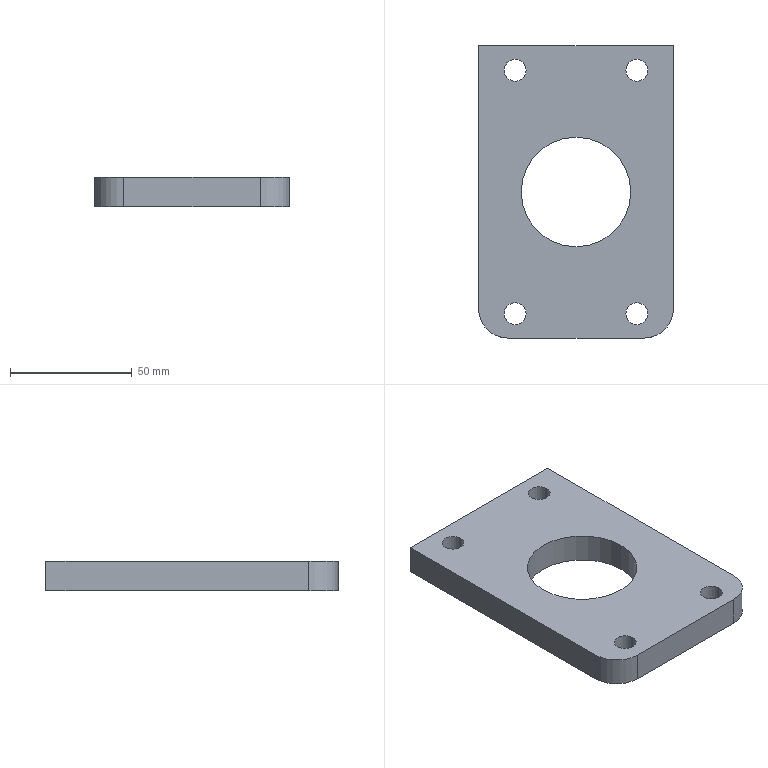Part | SolidWorks | features BaseBody 1 | 1 solid | 18 faces | box 80 x 120 x 12 mm | volume 92320 mm3 | cylinder 12 | plane 6 | commonest cylinder face diameters 9 x8 24 x2 45 x2
STEP:
#1=CARTESIAN_POINT('',(-255.5,-50.,-47.879));
#2=VERTEX_POINT('',#1);
#3=CARTESIAN_POINT('',(-264.5,-50.,-47.879));
#4=VERTEX_POINT('',#3);
#5=CARTESIAN_POINT('',(-260.,-50.,-47.879));
#6=DIRECTION('',(0.,0.,-1.));
#7=DIRECTION('',(-1.,0.,0.));
#8=AXIS2_PLACEMENT_3D('',#5,#6,#7);
#9=CIRCLE('',#8,4.5);
#10=EDGE_CURVE('',#2,#4,#9,.T.);
#11=ORIENTED_EDGE('',*,*,#10,.F.);
#12=CARTESIAN_POINT('',(-255.5,-50.,-59.879));
#13=VERTEX_POINT('',#12);
#14=CARTESIAN_POINT('',(-255.5,-50.,-59.879));
#15=DIRECTION('',(0.,0.,-1.));
#16=VECTOR('',#15,1000.);
#17=LINE('',#14,#16);
#18=EDGE_CURVE('',#2,#13,#17,.T.);
#19=ORIENTED_EDGE('',*,*,#18,.T.);
#20=CARTESIAN_POINT('',(-264.5,-50.,-59.879));
#21=VERTEX_POINT('',#20);
#22=CARTESIAN_POINT('',(-260.,-50.,-59.879));
#23=DIRECTION('',(0.,0.,1.));
#24=DIRECTION('',(-1.,0.,0.));
#25=AXIS2_PLACEMENT_3D('',#22,#23,#24);
#26=CIRCLE('',#25,4.5);
#27=EDGE_CURVE('',#21,#13,#26,.T.);
#28=ORIENTED_EDGE('',*,*,#27,.F.);
#29=CARTESIAN_POINT('',(-264.5,-50.,-59.879));
#30=DIRECTION('',(0.,0.,-1.));
#31=VECTOR('',#30,1000.);
#32=LINE('',#29,#31);
#33=EDGE_CURVE('',#4,#21,#32,.T.);
#34=ORIENTED_EDGE('',*,*,#33,.F.);
#35=EDGE_LOOP('',(#11,#19,#28,#34));
#36=FACE_OUTER_BOUND('',#35,.T.);
#37=CARTESIAN_POINT('',(-260.,-50.,-59.879));
#38=DIRECTION('',(0.,0.,-1.));
#39=DIRECTION('',(-1.,0.,0.));
#40=AXIS2_PLACEMENT_3D('',#37,#38,#39);
#41=CYLINDRICAL_SURFACE('',#40,4.5);
#42=ADVANCED_FACE('',(#36),#41,.F.);
#43=CARTESIAN_POINT('',(-205.5,-50.,-47.879));
#44=VERTEX_POINT('',#43);
#45=CARTESIAN_POINT('',(-214.5,-50.,-47.879));
#46=VERTEX_POINT('',#45);
#47=CARTESIAN_POINT('',(-210.,-50.,-47.879));
#48=DIRECTION('',(0.,0.,-1.));
#49=DIRECTION('',(-1.,0.,0.));
#50=AXIS2_PLACEMENT_3D('',#47,#48,#49);
#51=CIRCLE('',#50,4.5);
#52=EDGE_CURVE('',#44,#46,#51,.T.);
#53=ORIENTED_EDGE('',*,*,#52,.F.);
#54=CARTESIAN_POINT('',(-205.5,-50.,-59.879));
#55=VERTEX_POINT('',#54);
#56=CARTESIAN_POINT('',(-205.5,-50.,-59.879));
#57=DIRECTION('',(0.,0.,-1.));
#58=VECTOR('',#57,1000.);
#59=LINE('',#56,#58);
#60=EDGE_CURVE('',#44,#55,#59,.T.);
#61=ORIENTED_EDGE('',*,*,#60,.T.);
#62=CARTESIAN_POINT('',(-214.5,-50.,-59.879));
#63=VERTEX_POINT('',#62);
#64=CARTESIAN_POINT('',(-210.,-50.,-59.879));
#65=DIRECTION('',(0.,0.,1.));
#66=DIRECTION('',(-1.,0.,0.));
#67=AXIS2_PLACEMENT_3D('',#64,#65,#66);
#68=CIRCLE('',#67,4.5);
#69=EDGE_CURVE('',#63,#55,#68,.T.);
#70=ORIENTED_EDGE('',*,*,#69,.F.);
#71=CARTESIAN_POINT('',(-214.5,-50.,-59.879));
#72=DIRECTION('',(0.,0.,-1.));
#73=VECTOR('',#72,1000.);
#74=LINE('',#71,#73);
#75=EDGE_CURVE('',#46,#63,#74,.T.);
#76=ORIENTED_EDGE('',*,*,#75,.F.);
#77=EDGE_LOOP('',(#53,#61,#70,#76));
#78=FACE_OUTER_BOUND('',#77,.T.);
#79=CARTESIAN_POINT('',(-210.,-50.,-59.879));
#80=DIRECTION('',(0.,0.,-1.));
#81=DIRECTION('',(-1.,0.,0.));
#82=AXIS2_PLACEMENT_3D('',#79,#80,#81);
#83=CYLINDRICAL_SURFACE('',#82,4.5);
#84=ADVANCED_FACE('',(#78),#83,.F.);
#85=CARTESIAN_POINT('',(-212.5,0.,-47.879));
#86=VERTEX_POINT('',#85);
#87=CARTESIAN_POINT('',(-257.5,0.,-47.879));
#88=VERTEX_POINT('',#87);
#89=CARTESIAN_POINT('',(-235.,0.,-47.879));
#90=DIRECTION('',(0.,0.,-1.));
#91=DIRECTION('',(-1.,0.,0.));
#92=AXIS2_PLACEMENT_3D('',#89,#90,#91);
#93=CIRCLE('',#92,22.5);
#94=EDGE_CURVE('',#86,#88,#93,.T.);
#95=ORIENTED_EDGE('',*,*,#94,.F.);
#96=CARTESIAN_POINT('',(-212.5,0.,-59.879));
#97=VERTEX_POINT('',#96);
#98=CARTESIAN_POINT('',(-212.5,0.,-59.879));
#99=DIRECTION('',(0.,0.,-1.));
#100=VECTOR('',#99,1000.);
#101=LINE('',#98,#100);
#102=EDGE_CURVE('',#86,#97,#101,.T.);
#103=ORIENTED_EDGE('',*,*,#102,.T.);
#104=CARTESIAN_POINT('',(-257.5,0.,-59.879));
#105=VERTEX_POINT('',#104);
#106=CARTESIAN_POINT('',(-235.,0.,-59.879));
#107=DIRECTION('',(0.,0.,1.));
#108=DIRECTION('',(-1.,0.,0.));
#109=AXIS2_PLACEMENT_3D('',#106,#107,#108);
#110=CIRCLE('',#109,22.5);
#111=EDGE_CURVE('',#105,#97,#110,.T.);
#112=ORIENTED_EDGE('',*,*,#111,.F.);
#113=CARTESIAN_POINT('',(-257.5,0.,-59.879));
#114=DIRECTION('',(0.,0.,-1.));
#115=VECTOR('',#114,1000.);
#116=LINE('',#113,#115);
#117=EDGE_CURVE('',#88,#105,#116,.T.);
#118=ORIENTED_EDGE('',*,*,#117,.F.);
#119=EDGE_LOOP('',(#95,#103,#112,#118));
#120=FACE_OUTER_BOUND('',#119,.T.);
#121=CARTESIAN_POINT('',(-235.,0.,-59.879));
#122=DIRECTION('',(0.,0.,-1.));
#123=DIRECTION('',(-1.,0.,0.));
#124=AXIS2_PLACEMENT_3D('',#121,#122,#123);
#125=CYLINDRICAL_SURFACE('',#124,22.5);
#126=ADVANCED_FACE('',(#120),#125,.F.);
#127=CARTESIAN_POINT('',(-255.5,50.,-47.879));
#128=VERTEX_POINT('',#127);
#129=CARTESIAN_POINT('',(-264.5,50.,-47.879));
#130=VERTEX_POINT('',#129);
#131=CARTESIAN_POINT('',(-260.,50.,-47.879));
#132=DIRECTION('',(0.,0.,-1.));
#133=DIRECTION('',(-1.,0.,0.));
#134=AXIS2_PLACEMENT_3D('',#131,#132,#133);
#135=CIRCLE('',#134,4.5);
#136=EDGE_CURVE('',#128,#130,#135,.T.);
#137=ORIENTED_EDGE('',*,*,#136,.F.);
#138=CARTESIAN_POINT('',(-255.5,50.,-59.879));
#139=VERTEX_POINT('',#138);
#140=CARTESIAN_POINT('',(-255.5,50.,-59.879));
#141=DIRECTION('',(0.,0.,-1.));
#142=VECTOR('',#141,1000.);
#143=LINE('',#140,#142);
#144=EDGE_CURVE('',#128,#139,#143,.T.);
#145=ORIENTED_EDGE('',*,*,#144,.T.);
#146=CARTESIAN_POINT('',(-264.5,50.,-59.879));
#147=VERTEX_POINT('',#146);
#148=CARTESIAN_POINT('',(-260.,50.,-59.879));
#149=DIRECTION('',(0.,0.,1.));
#150=DIRECTION('',(-1.,0.,0.));
#151=AXIS2_PLACEMENT_3D('',#148,#149,#150);
#152=CIRCLE('',#151,4.5);
#153=EDGE_CURVE('',#147,#139,#152,.T.);
#154=ORIENTED_EDGE('',*,*,#153,.F.);
#155=CARTESIAN_POINT('',(-264.5,50.,-59.879));
#156=DIRECTION('',(0.,0.,-1.));
#157=VECTOR('',#156,1000.);
#158=LINE('',#155,#157);
#159=EDGE_CURVE('',#130,#147,#158,.T.);
#160=ORIENTED_EDGE('',*,*,#159,.F.);
#161=EDGE_LOOP('',(#137,#145,#154,#160));
#162=FACE_OUTER_BOUND('',#161,.T.);
#163=CARTESIAN_POINT('',(-260.,50.,-59.879));
#164=DIRECTION('',(0.,0.,-1.));
#165=DIRECTION('',(-1.,0.,0.));
#166=AXIS2_PLACEMENT_3D('',#163,#164,#165);
#167=CYLINDRICAL_SURFACE('',#166,4.5);
#168=ADVANCED_FACE('',(#162),#167,.F.);
#169=CARTESIAN_POINT('',(-205.5,50.,-47.879));
#170=VERTEX_POINT('',#169);
#171=CARTESIAN_POINT('',(-214.5,50.,-47.879));
#172=VERTEX_POINT('',#171);
#173=CARTESIAN_POINT('',(-210.,50.,-47.879));
#174=DIRECTION('',(0.,0.,-1.));
#175=DIRECTION('',(-1.,0.,0.));
#176=AXIS2_PLACEMENT_3D('',#173,#174,#175);
#177=CIRCLE('',#176,4.5);
#178=EDGE_CURVE('',#170,#172,#177,.T.);
#179=ORIENTED_EDGE('',*,*,#178,.F.);
#180=CARTESIAN_POINT('',(-205.5,50.,-59.879));
#181=VERTEX_POINT('',#180);
#182=CARTESIAN_POINT('',(-205.5,50.,-59.879));
#183=DIRECTION('',(0.,0.,-1.));
#184=VECTOR('',#183,1000.);
#185=LINE('',#182,#184);
#186=EDGE_CURVE('',#170,#181,#185,.T.);
#187=ORIENTED_EDGE('',*,*,#186,.T.);
#188=CARTESIAN_POINT('',(-214.5,50.,-59.879));
#189=VERTEX_POINT('',#188);
#190=CARTESIAN_POINT('',(-210.,50.,-59.879));
#191=DIRECTION('',(0.,0.,1.));
#192=DIRECTION('',(-1.,0.,0.));
#193=AXIS2_PLACEMENT_3D('',#190,#191,#192);
#194=CIRCLE('',#193,4.5);
#195=EDGE_CURVE('',#189,#181,#194,.T.);
#196=ORIENTED_EDGE('',*,*,#195,.F.);
#197=CARTESIAN_POINT('',(-214.5,50.,-59.879));
#198=DIRECTION('',(0.,0.,-1.));
#199=VECTOR('',#198,1000.);
#200=LINE('',#197,#199);
#201=EDGE_CURVE('',#172,#189,#200,.T.);
#202=ORIENTED_EDGE('',*,*,#201,.F.);
#203=EDGE_LOOP('',(#179,#187,#196,#202));
#204=FACE_OUTER_BOUND('',#203,.T.);
#205=CARTESIAN_POINT('',(-210.,50.,-59.879));
#206=DIRECTION('',(0.,0.,-1.));
#207=DIRECTION('',(-1.,0.,0.));
#208=AXIS2_PLACEMENT_3D('',#205,#206,#207);
#209=CYLINDRICAL_SURFACE('',#208,4.5);
#210=ADVANCED_FACE('',(#204),#209,.F.);
#211=CARTESIAN_POINT('',(-263.,-60.,-47.879));
#212=VERTEX_POINT('',#211);
#213=CARTESIAN_POINT('',(-207.,-60.,-47.879));
#214=VERTEX_POINT('',#213);
#215=CARTESIAN_POINT('',(-235.,-60.,-47.879));
#216=DIRECTION('',(1.,0.,0.));
#217=VECTOR('',#216,1000.);
#218=LINE('',#215,#217);
#219=EDGE_CURVE('',#212,#214,#218,.T.);
#220=ORIENTED_EDGE('',*,*,#219,.T.);
#221=CARTESIAN_POINT('',(-195.,-48.,-47.879));
#222=VERTEX_POINT('',#221);
#223=CARTESIAN_POINT('',(-207.,-48.,-47.879));
#224=DIRECTION('',(0.,0.,1.));
#225=DIRECTION('',(-1.,0.,0.));
#226=AXIS2_PLACEMENT_3D('',#223,#224,#225);
#227=CIRCLE('',#226,12.);
#228=EDGE_CURVE('',#214,#222,#227,.T.);
#229=ORIENTED_EDGE('',*,*,#228,.T.);
#230=CARTESIAN_POINT('',(-195.,60.,-47.879));
#231=VERTEX_POINT('',#230);
#232=CARTESIAN_POINT('',(-195.,0.,-47.879));
#233=DIRECTION('',(0.,1.,0.));
#234=VECTOR('',#233,1000.);
#235=LINE('',#232,#234);
#236=EDGE_CURVE('',#222,#231,#235,.T.);
#237=ORIENTED_EDGE('',*,*,#236,.T.);
#238=CARTESIAN_POINT('',(-275.,60.,-47.879));
#239=VERTEX_POINT('',#238);
#240=CARTESIAN_POINT('',(-235.,60.,-47.879));
#241=DIRECTION('',(-1.,0.,0.));
#242=VECTOR('',#241,1000.);
#243=LINE('',#240,#242);
#244=EDGE_CURVE('',#231,#239,#243,.T.);
#245=ORIENTED_EDGE('',*,*,#244,.T.);
#246=CARTESIAN_POINT('',(-275.,-48.,-47.879));
#247=VERTEX_POINT('',#246);
#248=CARTESIAN_POINT('',(-275.,0.,-47.879));
#249=DIRECTION('',(0.,-1.,0.));
#250=VECTOR('',#249,1000.);
#251=LINE('',#248,#250);
#252=EDGE_CURVE('',#239,#247,#251,.T.);
#253=ORIENTED_EDGE('',*,*,#252,.T.);
#254=CARTESIAN_POINT('',(-263.,-48.,-47.879));
#255=DIRECTION('',(0.,0.,1.));
#256=DIRECTION('',(-1.,0.,0.));
#257=AXIS2_PLACEMENT_3D('',#254,#255,#256);
#258=CIRCLE('',#257,12.);
#259=EDGE_CURVE('',#247,#212,#258,.T.);
#260=ORIENTED_EDGE('',*,*,#259,.T.);
#261=EDGE_LOOP('',(#220,#229,#237,#245,#253,#260));
#262=FACE_OUTER_BOUND('',#261,.T.);
#263=CARTESIAN_POINT('',(-260.,-50.,-47.879));
#264=DIRECTION('',(0.,0.,-1.));
#265=DIRECTION('',(-1.,0.,0.));
#266=AXIS2_PLACEMENT_3D('',#263,#264,#265);
#267=CIRCLE('',#266,4.5);
#268=EDGE_CURVE('',#4,#2,#267,.T.);
#269=ORIENTED_EDGE('',*,*,#268,.T.);
#270=ORIENTED_EDGE('',*,*,#10,.T.);
#271=EDGE_LOOP('',(#269,#270));
#272=FACE_BOUND('',#271,.T.);
#273=CARTESIAN_POINT('',(-210.,-50.,-47.879));
#274=DIRECTION('',(0.,0.,-1.));
#275=DIRECTION('',(-1.,0.,0.));
#276=AXIS2_PLACEMENT_3D('',#273,#274,#275);
#277=CIRCLE('',#276,4.5);
#278=EDGE_CURVE('',#46,#44,#277,.T.);
#279=ORIENTED_EDGE('',*,*,#278,.T.);
#280=ORIENTED_EDGE('',*,*,#52,.T.);
#281=EDGE_LOOP('',(#279,#280));
#282=FACE_BOUND('',#281,.T.);
#283=CARTESIAN_POINT('',(-235.,0.,-47.879));
#284=DIRECTION('',(0.,0.,-1.));
#285=DIRECTION('',(-1.,0.,0.));
#286=AXIS2_PLACEMENT_3D('',#283,#284,#285);
#287=CIRCLE('',#286,22.5);
#288=EDGE_CURVE('',#88,#86,#287,.T.);
#289=ORIENTED_EDGE('',*,*,#288,.T.);
#290=ORIENTED_EDGE('',*,*,#94,.T.);
#291=EDGE_LOOP('',(#289,#290));
#292=FACE_BOUND('',#291,.T.);
#293=CARTESIAN_POINT('',(-260.,50.,-47.879));
#294=DIRECTION('',(0.,0.,-1.));
#295=DIRECTION('',(-1.,0.,0.));
#296=AXIS2_PLACEMENT_3D('',#293,#294,#295);
#297=CIRCLE('',#296,4.5);
#298=EDGE_CURVE('',#130,#128,#297,.T.);
#299=ORIENTED_EDGE('',*,*,#298,.T.);
#300=ORIENTED_EDGE('',*,*,#136,.T.);
#301=EDGE_LOOP('',(#299,#300));
#302=FACE_BOUND('',#301,.T.);
#303=CARTESIAN_POINT('',(-210.,50.,-47.879));
#304=DIRECTION('',(0.,0.,-1.));
#305=DIRECTION('',(-1.,0.,0.));
#306=AXIS2_PLACEMENT_3D('',#303,#304,#305);
#307=CIRCLE('',#306,4.5);
#308=EDGE_CURVE('',#172,#170,#307,.T.);
#309=ORIENTED_EDGE('',*,*,#308,.T.);
#310=ORIENTED_EDGE('',*,*,#178,.T.);
#311=EDGE_LOOP('',(#309,#310));
#312=FACE_BOUND('',#311,.T.);
#313=CARTESIAN_POINT('',(-235.,0.,-47.879));
#314=DIRECTION('',(0.,0.,1.));
#315=DIRECTION('',(1.,0.,0.));
#316=AXIS2_PLACEMENT_3D('',#313,#314,#315);
#317=PLANE('',#316);
#318=ADVANCED_FACE('',(#262,#272,#282,#292,#302,#312),#317,.T.);
#319=ORIENTED_EDGE('',*,*,#228,.F.);
#320=CARTESIAN_POINT('',(-207.,-60.,-59.879));
#321=VERTEX_POINT('',#320);
#322=CARTESIAN_POINT('',(-207.,-60.,-59.879));
#323=DIRECTION('',(0.,0.,-1.));
#324=VECTOR('',#323,1000.);
#325=LINE('',#322,#324);
#326=EDGE_CURVE('',#214,#321,#325,.T.);
#327=ORIENTED_EDGE('',*,*,#326,.T.);
#328=CARTESIAN_POINT('',(-195.,-48.,-59.879));
#329=VERTEX_POINT('',#328);
#330=CARTESIAN_POINT('',(-207.,-48.,-59.879));
#331=DIRECTION('',(0.,0.,1.));
#332=DIRECTION('',(-1.,0.,0.));
#333=AXIS2_PLACEMENT_3D('',#330,#331,#332);
#334=CIRCLE('',#333,12.);
#335=EDGE_CURVE('',#321,#329,#334,.T.);
#336=ORIENTED_EDGE('',*,*,#335,.T.);
#337=CARTESIAN_POINT('',(-195.,-48.,-59.879));
#338=DIRECTION('',(0.,0.,1.));
#339=VECTOR('',#338,1000.);
#340=LINE('',#337,#339);
#341=EDGE_CURVE('',#329,#222,#340,.T.);
#342=ORIENTED_EDGE('',*,*,#341,.T.);
#343=EDGE_LOOP('',(#319,#327,#336,#342));
#344=FACE_OUTER_BOUND('',#343,.T.);
#345=CARTESIAN_POINT('',(-207.,-48.,-59.879));
#346=DIRECTION('',(0.,0.,-1.));
#347=DIRECTION('',(-1.,0.,0.));
#348=AXIS2_PLACEMENT_3D('',#345,#346,#347);
#349=CYLINDRICAL_SURFACE('',#348,12.);
#350=ADVANCED_FACE('',(#344),#349,.T.);
#351=ORIENTED_EDGE('',*,*,#219,.F.);
#352=CARTESIAN_POINT('',(-263.,-60.,-59.879));
#353=VERTEX_POINT('',#352);
#354=CARTESIAN_POINT('',(-263.,-60.,-59.879));
#355=DIRECTION('',(0.,0.,-1.));
#356=VECTOR('',#355,1000.);
#357=LINE('',#354,#356);
#358=EDGE_CURVE('',#212,#353,#357,.T.);
#359=ORIENTED_EDGE('',*,*,#358,.T.);
#360=CARTESIAN_POINT('',(-207.,-60.,-59.879));
#361=DIRECTION('',(1.,0.,0.));
#362=VECTOR('',#361,1000.);
#363=LINE('',#360,#362);
#364=EDGE_CURVE('',#353,#321,#363,.T.);
#365=ORIENTED_EDGE('',*,*,#364,.T.);
#366=ORIENTED_EDGE('',*,*,#326,.F.);
#367=EDGE_LOOP('',(#351,#359,#365,#366));
#368=FACE_OUTER_BOUND('',#367,.T.);
#369=CARTESIAN_POINT('',(-207.,-60.,-59.879));
#370=DIRECTION('',(0.,-1.,0.));
#371=DIRECTION('',(0.,0.,-1.));
#372=AXIS2_PLACEMENT_3D('',#369,#370,#371);
#373=PLANE('',#372);
#374=ADVANCED_FACE('',(#368),#373,.T.);
#375=ORIENTED_EDGE('',*,*,#259,.F.);
#376=CARTESIAN_POINT('',(-275.,-48.,-59.879));
#377=VERTEX_POINT('',#376);
#378=CARTESIAN_POINT('',(-275.,-48.,-59.879));
#379=DIRECTION('',(0.,0.,-1.));
#380=VECTOR('',#379,1000.);
#381=LINE('',#378,#380);
#382=EDGE_CURVE('',#247,#377,#381,.T.);
#383=ORIENTED_EDGE('',*,*,#382,.T.);
#384=CARTESIAN_POINT('',(-263.,-48.,-59.879));
#385=DIRECTION('',(0.,0.,1.));
#386=DIRECTION('',(-1.,0.,0.));
#387=AXIS2_PLACEMENT_3D('',#384,#385,#386);
#388=CIRCLE('',#387,12.);
#389=EDGE_CURVE('',#377,#353,#388,.T.);
#390=ORIENTED_EDGE('',*,*,#389,.T.);
#391=ORIENTED_EDGE('',*,*,#358,.F.);
#392=EDGE_LOOP('',(#375,#383,#390,#391));
#393=FACE_OUTER_BOUND('',#392,.T.);
#394=CARTESIAN_POINT('',(-263.,-48.,-59.879));
#395=DIRECTION('',(0.,0.,-1.));
#396=DIRECTION('',(-1.,0.,0.));
#397=AXIS2_PLACEMENT_3D('',#394,#395,#396);
#398=CYLINDRICAL_SURFACE('',#397,12.);
#399=ADVANCED_FACE('',(#393),#398,.T.);
#400=ORIENTED_EDGE('',*,*,#252,.F.);
#401=CARTESIAN_POINT('',(-275.,60.,-59.879));
#402=VERTEX_POINT('',#401);
#403=CARTESIAN_POINT('',(-275.,60.,-59.879));
#404=DIRECTION('',(0.,0.,-1.));
#405=VECTOR('',#404,1000.);
#406=LINE('',#403,#405);
#407=EDGE_CURVE('',#239,#402,#406,.T.);
#408=ORIENTED_EDGE('',*,*,#407,.T.);
#409=CARTESIAN_POINT('',(-275.,-48.,-59.879));
#410=DIRECTION('',(0.,-1.,0.));
#411=VECTOR('',#410,1000.);
#412=LINE('',#409,#411);
#413=EDGE_CURVE('',#402,#377,#412,.T.);
#414=ORIENTED_EDGE('',*,*,#413,.T.);
#415=ORIENTED_EDGE('',*,*,#382,.F.);
#416=EDGE_LOOP('',(#400,#408,#414,#415));
#417=FACE_OUTER_BOUND('',#416,.T.);
#418=CARTESIAN_POINT('',(-275.,-48.,-59.879));
#419=DIRECTION('',(-1.,0.,0.));
#420=DIRECTION('',(0.,0.,1.));
#421=AXIS2_PLACEMENT_3D('',#418,#419,#420);
#422=PLANE('',#421);
#423=ADVANCED_FACE('',(#417),#422,.T.);
#424=ORIENTED_EDGE('',*,*,#244,.F.);
#425=CARTESIAN_POINT('',(-195.,60.,-59.879));
#426=VERTEX_POINT('',#425);
#427=CARTESIAN_POINT('',(-195.,60.,-59.879));
#428=DIRECTION('',(0.,0.,-1.));
#429=VECTOR('',#428,1000.);
#430=LINE('',#427,#429);
#431=EDGE_CURVE('',#231,#426,#430,.T.);
#432=ORIENTED_EDGE('',*,*,#431,.T.);
#433=CARTESIAN_POINT('',(-263.,60.,-59.879));
#434=DIRECTION('',(-1.,0.,0.));
#435=VECTOR('',#434,1000.);
#436=LINE('',#433,#435);
#437=EDGE_CURVE('',#426,#402,#436,.T.);
#438=ORIENTED_EDGE('',*,*,#437,.T.);
#439=ORIENTED_EDGE('',*,*,#407,.F.);
#440=EDGE_LOOP('',(#424,#432,#438,#439));
#441=FACE_OUTER_BOUND('',#440,.T.);
#442=CARTESIAN_POINT('',(-263.,60.,-59.879));
#443=DIRECTION('',(0.,1.,0.));
#444=DIRECTION('',(0.,0.,1.));
#445=AXIS2_PLACEMENT_3D('',#442,#443,#444);
#446=PLANE('',#445);
#447=ADVANCED_FACE('',(#441),#446,.T.);
#448=ORIENTED_EDGE('',*,*,#236,.F.);
#449=ORIENTED_EDGE('',*,*,#341,.F.);
#450=CARTESIAN_POINT('',(-195.,48.,-59.879));
#451=DIRECTION('',(0.,1.,0.));
#452=VECTOR('',#451,1000.);
#453=LINE('',#450,#452);
#454=EDGE_CURVE('',#329,#426,#453,.T.);
#455=ORIENTED_EDGE('',*,*,#454,.T.);
#456=ORIENTED_EDGE('',*,*,#431,.F.);
#457=EDGE_LOOP('',(#448,#449,#455,#456));
#458=FACE_OUTER_BOUND('',#457,.T.);
#459=CARTESIAN_POINT('',(-195.,48.,-59.879));
#460=DIRECTION('',(1.,0.,0.));
#461=DIRECTION('',(0.,0.,-1.));
#462=AXIS2_PLACEMENT_3D('',#459,#460,#461);
#463=PLANE('',#462);
#464=ADVANCED_FACE('',(#458),#463,.T.);
#465=ORIENTED_EDGE('',*,*,#18,.F.);
#466=ORIENTED_EDGE('',*,*,#268,.F.);
#467=ORIENTED_EDGE('',*,*,#33,.T.);
#468=CARTESIAN_POINT('',(-260.,-50.,-59.879));
#469=DIRECTION('',(0.,0.,1.));
#470=DIRECTION('',(-1.,0.,0.));
#471=AXIS2_PLACEMENT_3D('',#468,#469,#470);
#472=CIRCLE('',#471,4.5);
#473=EDGE_CURVE('',#13,#21,#472,.T.);
#474=ORIENTED_EDGE('',*,*,#473,.F.);
#475=EDGE_LOOP('',(#465,#466,#467,#474));
#476=FACE_OUTER_BOUND('',#475,.T.);
#477=CARTESIAN_POINT('',(-260.,-50.,-59.879));
#478=DIRECTION('',(0.,0.,-1.));
#479=DIRECTION('',(-1.,0.,0.));
#480=AXIS2_PLACEMENT_3D('',#477,#478,#479);
#481=CYLINDRICAL_SURFACE('',#480,4.5);
#482=ADVANCED_FACE('',(#476),#481,.F.);
#483=ORIENTED_EDGE('',*,*,#60,.F.);
#484=ORIENTED_EDGE('',*,*,#278,.F.);
#485=ORIENTED_EDGE('',*,*,#75,.T.);
#486=CARTESIAN_POINT('',(-210.,-50.,-59.879));
#487=DIRECTION('',(0.,0.,1.));
#488=DIRECTION('',(-1.,0.,0.));
#489=AXIS2_PLACEMENT_3D('',#486,#487,#488);
#490=CIRCLE('',#489,4.5);
#491=EDGE_CURVE('',#55,#63,#490,.T.);
#492=ORIENTED_EDGE('',*,*,#491,.F.);
#493=EDGE_LOOP('',(#483,#484,#485,#492));
#494=FACE_OUTER_BOUND('',#493,.T.);
#495=CARTESIAN_POINT('',(-210.,-50.,-59.879));
#496=DIRECTION('',(0.,0.,-1.));
#497=DIRECTION('',(-1.,0.,0.));
#498=AXIS2_PLACEMENT_3D('',#495,#496,#497);
#499=CYLINDRICAL_SURFACE('',#498,4.5);
#500=ADVANCED_FACE('',(#494),#499,.F.);
#501=ORIENTED_EDGE('',*,*,#102,.F.);
#502=ORIENTED_EDGE('',*,*,#288,.F.);
#503=ORIENTED_EDGE('',*,*,#117,.T.);
#504=CARTESIAN_POINT('',(-235.,0.,-59.879));
#505=DIRECTION('',(0.,0.,1.));
#506=DIRECTION('',(-1.,0.,0.));
#507=AXIS2_PLACEMENT_3D('',#504,#505,#506);
#508=CIRCLE('',#507,22.5);
#509=EDGE_CURVE('',#97,#105,#508,.T.);
#510=ORIENTED_EDGE('',*,*,#509,.F.);
#511=EDGE_LOOP('',(#501,#502,#503,#510));
#512=FACE_OUTER_BOUND('',#511,.T.);
#513=CARTESIAN_POINT('',(-235.,0.,-59.879));
#514=DIRECTION('',(0.,0.,-1.));
#515=DIRECTION('',(-1.,0.,0.));
#516=AXIS2_PLACEMENT_3D('',#513,#514,#515);
#517=CYLINDRICAL_SURFACE('',#516,22.5);
#518=ADVANCED_FACE('',(#512),#517,.F.);
#519=ORIENTED_EDGE('',*,*,#144,.F.);
#520=ORIENTED_EDGE('',*,*,#298,.F.);
#521=ORIENTED_EDGE('',*,*,#159,.T.);
#522=CARTESIAN_POINT('',(-260.,50.,-59.879));
#523=DIRECTION('',(0.,0.,1.));
#524=DIRECTION('',(-1.,0.,0.));
#525=AXIS2_PLACEMENT_3D('',#522,#523,#524);
#526=CIRCLE('',#525,4.5);
#527=EDGE_CURVE('',#139,#147,#526,.T.);
#528=ORIENTED_EDGE('',*,*,#527,.F.);
#529=EDGE_LOOP('',(#519,#520,#521,#528));
#530=FACE_OUTER_BOUND('',#529,.T.);
#531=CARTESIAN_POINT('',(-260.,50.,-59.879));
#532=DIRECTION('',(0.,0.,-1.));
#533=DIRECTION('',(-1.,0.,0.));
#534=AXIS2_PLACEMENT_3D('',#531,#532,#533);
#535=CYLINDRICAL_SURFACE('',#534,4.5);
#536=ADVANCED_FACE('',(#530),#535,.F.);
#537=ORIENTED_EDGE('',*,*,#186,.F.);
#538=ORIENTED_EDGE('',*,*,#308,.F.);
#539=ORIENTED_EDGE('',*,*,#201,.T.);
#540=CARTESIAN_POINT('',(-210.,50.,-59.879));
#541=DIRECTION('',(0.,0.,1.));
#542=DIRECTION('',(-1.,0.,0.));
#543=AXIS2_PLACEMENT_3D('',#540,#541,#542);
#544=CIRCLE('',#543,4.5);
#545=EDGE_CURVE('',#181,#189,#544,.T.);
#546=ORIENTED_EDGE('',*,*,#545,.F.);
#547=EDGE_LOOP('',(#537,#538,#539,#546));
#548=FACE_OUTER_BOUND('',#547,.T.);
#549=CARTESIAN_POINT('',(-210.,50.,-59.879));
#550=DIRECTION('',(0.,0.,-1.));
#551=DIRECTION('',(-1.,0.,0.));
#552=AXIS2_PLACEMENT_3D('',#549,#550,#551);
#553=CYLINDRICAL_SURFACE('',#552,4.5);
#554=ADVANCED_FACE('',(#548),#553,.F.);
#555=ORIENTED_EDGE('',*,*,#454,.F.);
#556=ORIENTED_EDGE('',*,*,#335,.F.);
#557=ORIENTED_EDGE('',*,*,#364,.F.);
#558=ORIENTED_EDGE('',*,*,#389,.F.);
#559=ORIENTED_EDGE('',*,*,#413,.F.);
#560=ORIENTED_EDGE('',*,*,#437,.F.);
#561=EDGE_LOOP('',(#555,#556,#557,#558,#559,#560));
#562=FACE_OUTER_BOUND('',#561,.T.);
#563=ORIENTED_EDGE('',*,*,#27,.T.);
#564=ORIENTED_EDGE('',*,*,#473,.T.);
#565=EDGE_LOOP('',(#563,#564));
#566=FACE_BOUND('',#565,.T.);
#567=ORIENTED_EDGE('',*,*,#69,.T.);
#568=ORIENTED_EDGE('',*,*,#491,.T.);
#569=EDGE_LOOP('',(#567,#568));
#570=FACE_BOUND('',#569,.T.);
#571=ORIENTED_EDGE('',*,*,#111,.T.);
#572=ORIENTED_EDGE('',*,*,#509,.T.);
#573=EDGE_LOOP('',(#571,#572));
#574=FACE_BOUND('',#573,.T.);
#575=ORIENTED_EDGE('',*,*,#153,.T.);
#576=ORIENTED_EDGE('',*,*,#527,.T.);
#577=EDGE_LOOP('',(#575,#576));
#578=FACE_BOUND('',#577,.T.);
#579=ORIENTED_EDGE('',*,*,#195,.T.);
#580=ORIENTED_EDGE('',*,*,#545,.T.);
#581=EDGE_LOOP('',(#579,#580));
#582=FACE_BOUND('',#581,.T.);
#583=CARTESIAN_POINT('',(-235.,0.,-59.879));
#584=DIRECTION('',(0.,0.,1.));
#585=DIRECTION('',(1.,0.,0.));
#586=AXIS2_PLACEMENT_3D('',#583,#584,#585);
#587=PLANE('',#586);
#588=ADVANCED_FACE('',(#562,#566,#570,#574,#578,#582),#587,.F.);
#589=CLOSED_SHELL('',(#42,#84,#126,#168,#210,#318,#350,#374,#399,#423,#447,#464,#482,#500,#518,#536,#554,#588));
#590=MANIFOLD_SOLID_BREP('',#589);
#591=CARTESIAN_POINT('',(0.,0.,0.));
#592=DIRECTION('',(0.,0.,1.));
#593=DIRECTION('',(1.,0.,0.));
#594=AXIS2_PLACEMENT_3D('',#591,#592,#593);
#595=(LENGTH_UNIT()NAMED_UNIT(*)SI_UNIT(.MILLI.,.METRE.));
#596=UNCERTAINTY_MEASURE_WITH_UNIT(LENGTH_MEASURE(0.00001),#595,'','');
#597=(NAMED_UNIT(*)PLANE_ANGLE_UNIT()SI_UNIT($,.RADIAN.));
#598=(NAMED_UNIT(*)SI_UNIT($,.STERADIAN.)SOLID_ANGLE_UNIT());
#599=(GEOMETRIC_REPRESENTATION_CONTEXT(3)GLOBAL_UNCERTAINTY_ASSIGNED_CONTEXT((#596))GLOBAL_UNIT_ASSIGNED_CONTEXT((#595,#597,#598))REPRESENTATION_CONTEXT('',''));
#600=ADVANCED_BREP_SHAPE_REPRESENTATION('',(#590,#594),#599);